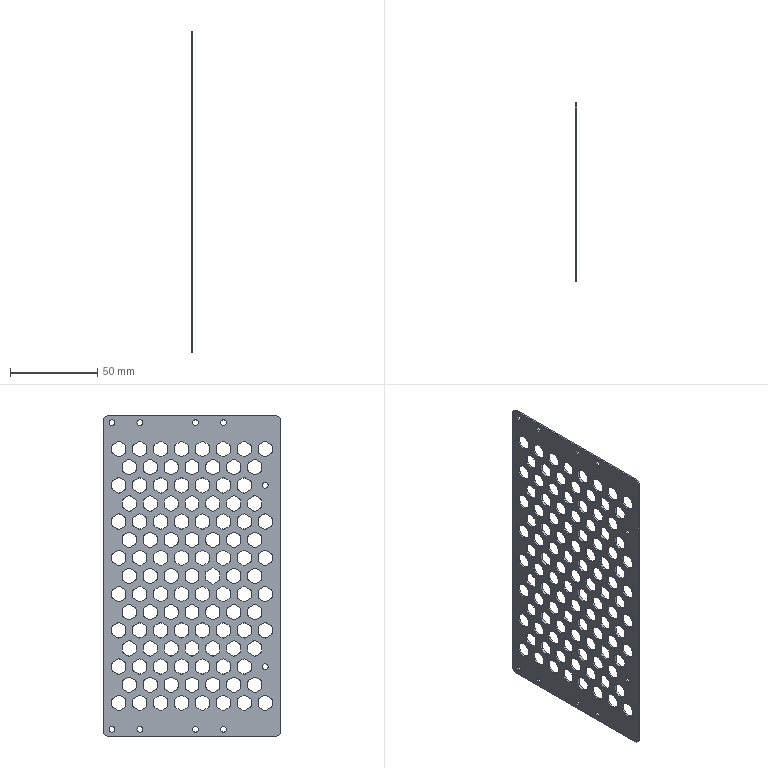Part | SolidWorks | features Fillet 2, ICE 2, APattern 1, Extrusion 1 | 1 solid | 1466 faces | box 1 x 101.95 x 184 mm | volume 12597 mm3 | cylinder 794 | plane 672 | commonest cylinder face diameters 3 x770 3.2 x16 3.3 x4 6 x4